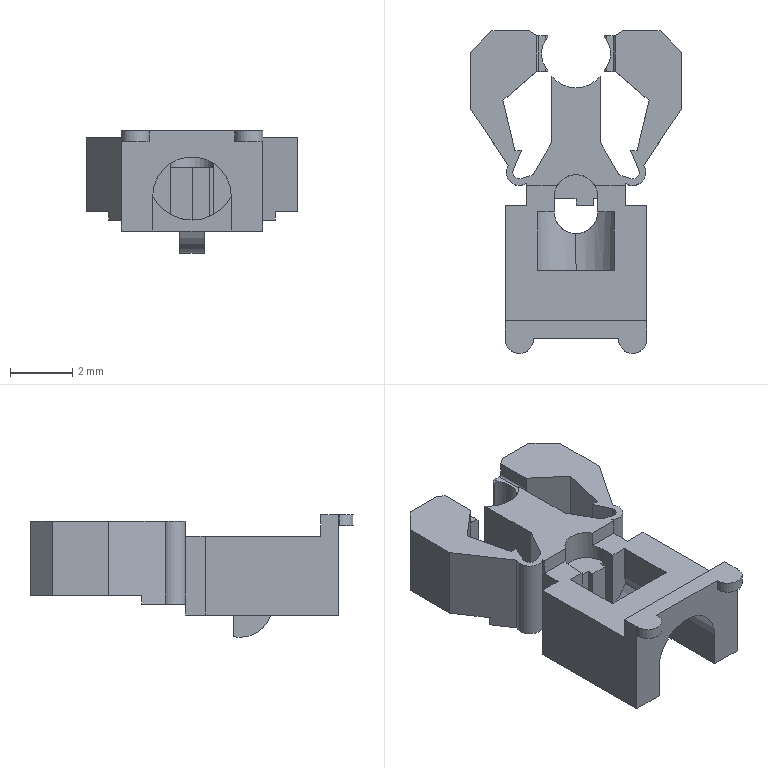Part | SolidWorks | features ICE 21, MirrorPattern 4, Chamfer 2, MoveFace 2, Extrusion 1, Fillet 1, Scale 1 | 1 solid | 117 faces | box 6.79 x 10.36 x 3.938 mm | volume 78.166 mm3 | plane 91 | cylinder 26 | commonest cylinder face diameters 0.91 x6 0.14 x4 0.42 x3 0.84 x3 1.52 x3 1.4 x2